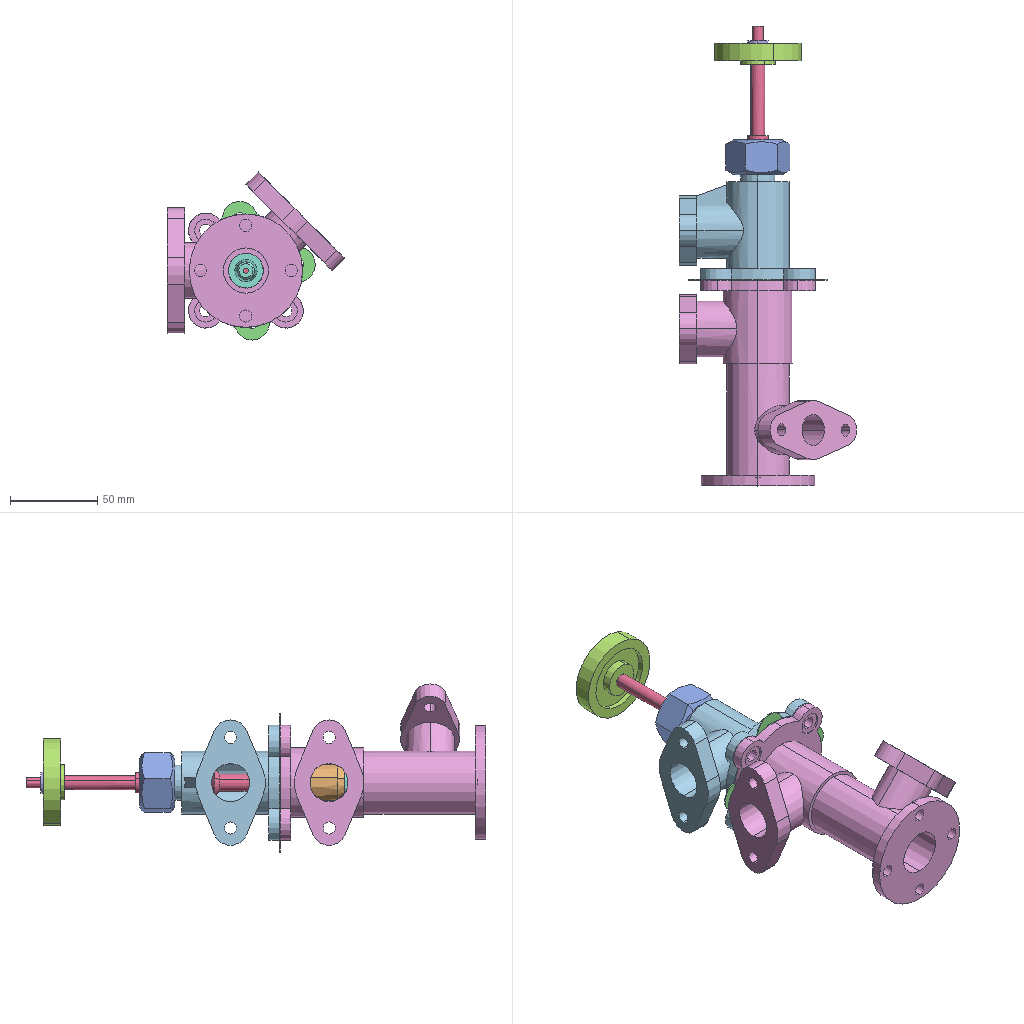Assembly | SolidWorks | 10 different items | 10 placed | box 102 x 264 x 96 mm
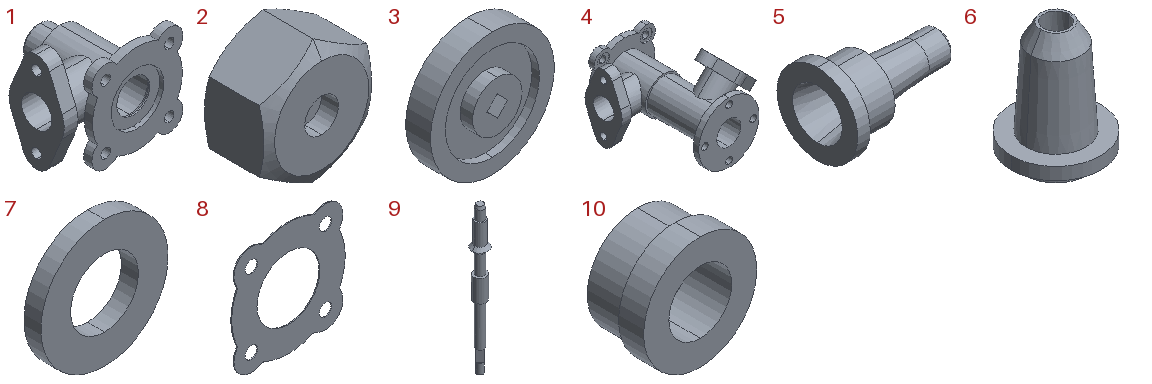Parts list (item | quantity | size | volume | features):
1 | x1 | 77.981 x 72 x 72 mm | 74377 mm3 | features ICE 13, Chamfer 2, Extrusion 1, Fillet 1, Rib 1, StudWizard 1
2 | x1 | 32 x 20 x 36.95 mm | 13532 mm3 | features ICE 2, Extrusion 1, MirrorPattern 1, RevCut 1
3 | x1 | 50 x 12 x 50 mm | 14912 mm3 | features ICE 3, Extrusion 1
4 | x1 | 101.569 x 118 x 92.569 mm | 130273 mm3 | features ICE 20, Extrusion 1
5 | x1 | 39 x 26 x 26 mm | 5238 mm3 | features Chamfer 1, Extrusion 1, RevCut 1, Revolution 1
6 | x1 | 36 x 36 x 48 mm | 14193 mm3 | features Extrusion 1, ICE 1, RevCut 1, Revolution 1
7 | x1 | 12 x 1.6 x 12 mm | 129.484 mm3 | features Extrusion 1
8 | x1 | 65 x 0.5 x 65 mm | 1310 mm3 | features Extrusion 1, Fillet 1, ICE 1
9 | x1 | 16 x 16 x 145 mm | 9307 mm3 | features ICE 8, Chamfer 3, Extrusion 1
10 | x1 | 18 x 10 x 18 mm | 1269 mm3 | features ICE 2, Chamfer 1, Extrusion 1
Mates (type | each side: item.copy, entity, surface, feature):
Coincident | 4.1 plane | assembly plane | 3 times
Concentric | 4.1 face cylinder Cut-Extrude5 | 9.1 face cylinder Boss-Extrude3
Concentric | 5.1 face cone Cut-Revolve1 | 9.1 face cylinder Boss-Extrude7
Concentric | 4.1 face cylinder Cut-Extrude5 | 8.1 face cylinder Cut-Extrude1
Coincident | 4.1 face plane Boss-Extrude3 | 8.1 face plane Boss-Extrude1
Tangent | 4.1 face cylinder Boss-Extrude4 | 8.1 face cylinder Boss-Extrude1 | 2 times
Concentric | 4.1 face cylinder Cut-Extrude5 | 1.1 face cylinder Cut-Extrude3
Concentric | 4.1 face cylinder Cut-Extrude7 | 1.1 face cylinder Cut-Extrude8
Coincident | 8.1 face plane Boss-Extrude1 | 1.1 face plane Boss-Extrude1
Concentric | 2.1 face cylinder Cut-Extrude1 | 1.1 face cylinder Cut-Extrude6
Coincident | 3.1 face plane Cut-Extrude1 | 9.1 face plane Cut-Extrude1 | 2 times
Concentric | 4.1 face cylinder Cut-Extrude1 | 6.1 face cone Cut-Revolve1
Coincident | 4.1 face plane Cut-Extrude4 | 6.1 face plane Boss-Extrude2
Coincident | 4.1 face plane Cut-Extrude6 | 5.1 face plane Revolve1
Concentric | 10.1 face cylinder Cut-Extrude1 | 1.1 face cylinder Boss-Extrude3
Coincident | 3.1 face plane Boss-Extrude2 | 9.1 face plane Cut-Extrude1
Concentric | 7.1 face cylinder Boss-Extrude1 | 9.1 face cylinder Boss-Extrude1
Coincident | 3.1 face plane Boss-Extrude2 | 7.1 face plane Boss-Extrude1
Coincident | 10.1 face plane Boss-Extrude1 | 2.1 face plane Cut-Extrude2
Coincident | 2.1 face plane Boss-Extrude1 | 1.1 face plane Boss-Extrude4